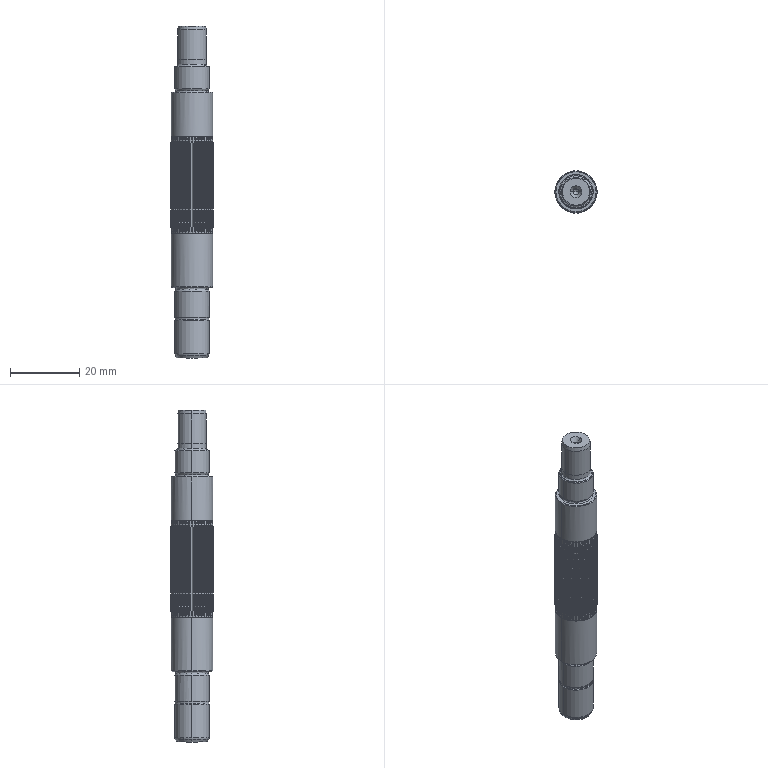Part | STEP file | TQ-DD-1105-THShaft1010_デフォルト | 1 solid | 390 faces | box 12.206 x 12.206 x 96.2 mm | volume 9184 mm3 | plane 165 | cylinder 109 | cone 104 | spline 12 | commonest cylinder face diameters 0.18 x49 12.22 x40 1.6 x4 10 x4 12 x4 8.25 x2